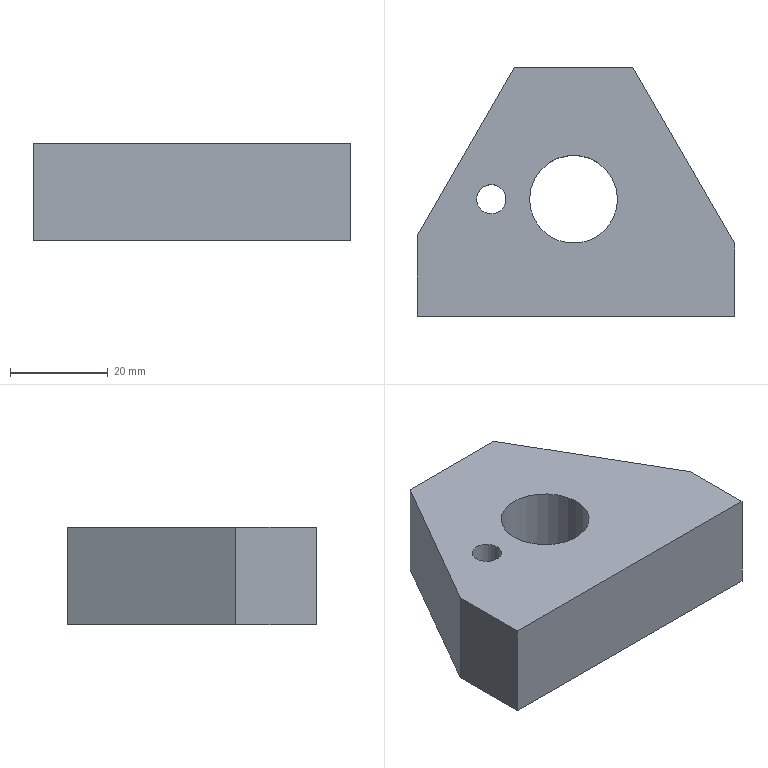NC program | NX | posted with a generic post | part box 65 x 51 x 20 mm
Whole program, first 1325 of 1400 lines:
N10 G17 G21 G94 G90
(ADAPTIVE_MILLING , TOOL : D8)
N12 T02 M6
N14 G53
N16 G17 G0 G90 X12.189 Y36.097 B0. C0. S5500 M3
N18 G43 Z30.2 H2
N20 Z3.
N22 G94 G1 X12.207 Y35.949 Z2.063 F2500.
N24 X12.226 Y35.8 Z1.692
N26 X12.244 Y35.651 Z1.42
N28 X12.263 Y35.502 Z1.2
N30 X12.282 Y35.353 Z1.016
N32 X12.3 Y35.204 Z0.858
N34 X12.319 Y35.056 Z0.72
N36 X12.338 Y34.907 Z0.6
N38 X12.356 Y34.758 Z0.495
N40 X12.375 Y34.609 Z0.402
N42 X12.393 Y34.46 Z0.321
N44 X12.412 Y34.311 Z0.25
N46 X12.431 Y34.163 Z0.19
N48 X12.449 Y34.014 Z0.138
N50 X12.468 Y33.865 Z0.095
N52 X12.487 Y33.716 Z0.061
N54 X12.505 Y33.567 Z0.034
N56 X12.524 Y33.418 Z0.015
N58 X12.542 Y33.27 Z0.004
N60 X12.561 Y33.121 Z0.
N62 X12.741 Y31.68
N64 G3 X13.293 Y31.012 R0.809
N66 X15.497 Y30.394 R12.881
N68 X21.026 Y30.043 R42.106
N70 X30.728 Y29.99 R751.289
N72 G2 X33.593 Y28.371 R4.374
N74 X35.342 Y24.592 R8.747
N76 X35.918 Y19.006 R30.143
N78 X36. Y6.781 R494.796
N80 G1 X36.013 Y-5.87
N82 X36.085 Y-6.101
N84 G2 X36.947 Y-7.722 R12.356
N86 G1 X37.005 Y-7.94
N88 G3 X36.638 Y-7.058 R3.65
N90 G2 X35.94 Y-5.799 R10.806
N92 X35.519 Y-2.949 R11.424
N94 X35.401 Y4.651 R164.559
N96 G3 X35.308 Y18.774 R515.844
N98 X34.731 Y23.984 R26.878
N100 X33.536 Y26.625 R6.339
N102 X30.052 Y28.714 R6.857
N104 X25.302 Y29.326 R21.254
N106 G2 X18.159 Y29.565 R325.443
N108 X15.126 Y29.981 R16.107
N110 X14.593 Y30.398 R2.093
N112 G1 X13.833 Y30.837
N114 G2 X15.21 Y29.843 R4.704
N116 G3 X17.513 Y28.97 R6.034
N118 X22.406 Y28.472 R34.474
N120 G2 X27.483 Y28.063 R46.592
N122 X30.66 Y26.815 R6.875
N124 X33.235 Y23.022 R8.035
N126 X34.172 Y17.947 R20.137
N128 X34.393 Y8.877 R133.127
N130 G3 X34.49 Y-1.554 R317.27
N132 X34.67 Y-3.615 R16.857
N134 X36.025 Y-5.998 R47.331
N136 G1 X34.529 Y-3.374
N138 G2 X33.982 Y-0.466 R10.299
N140 X33.799 Y7.21 R114.665
N142 G3 X33.62 Y16.757 R176.883
N144 X32.766 Y21.999 R21.482
N146 X28.366 Y26.699 R7.128
N148 X23.91 Y27.672 R17.04
N150 G2 X18.768 Y28.21 R116.087
N152 X15.92 Y29.009 R10.067
N154 G1 X15.689 Y29.199
N156 X15.19 Y29.861
N158 X15.985 Y28.817
N160 G3 X18.181 Y27.684 R5.485
N162 X22.159 Y26.925 R27.744
N164 G2 X26.35 Y26.099 R24.625
N166 X31.006 Y21.977 R7.689
N168 X32.391 Y16.852 R16.158
N170 X32.767 Y9.59 R68.766
N172 G3 X32.931 Y1.036 R215.232
N174 X33.136 Y-0.96 R18.787
N176 X34.601 Y-3.531 R124.339
N178 G1 X32.988 Y-0.707
N180 G2 X32.409 Y2.188 R10.174
N182 X32.172 Y9.2 R107.328
N184 G3 X31.756 Y16.609 R64.499
N186 X30.392 Y21.342 R14.403
N188 X26.079 Y25.131 R8.196
N190 X21.958 Y26.26 R22.038
N192 G2 X17.969 Y27.237 R27.216
N194 X16.373 Y28.082 R5.11
N196 X15.763 Y29.097 R13.29
N198 G3 X16.568 Y27.739 R54.163
N200 X18.642 Y26.378 R5.292
N202 X22.56 Y25.167 R37.442
N204 G2 X26.34 Y23.545 R12.816
N206 X29.729 Y19.042 R9.389
N208 X30.904 Y13.329 R21.33
N210 X31.243 Y5.627 R145.237
N212 G3 X31.537 Y1.832 R35.701
N214 G1 X31.591 Y1.683
N216 X33.091 Y-0.915
N218 X31.406 Y2.027
N220 G2 X30.803 Y4.924 R10.206
N222 X30.43 Y11.325 R214.4
N224 G3 X29.565 Y17.175 R28.198
N226 X26.97 Y21.765 R10.057
N228 X22.872 Y24.225 R12.042
N230 G2 X19.002 Y25.654 R134.738
N232 X17.185 Y26.687 R7.855
N234 X16.451 Y27.906 R10.718
N236 G1 X17.393 Y26.302
N238 G3 X19.431 Y24.779 R6.287
N240 G1 X22.915 Y23.099
N242 G2 X28.116 Y17.11 R10.513
N244 X29.303 Y11.315 R23.654
N246 G3 X29.808 Y5.321 R379.785
N248 X29.965 Y4.5 R3.274
N250 G1 X31.502 Y1.837
N252 X29.747 Y4.904
N254 G2 X29.095 Y7.836 R11.845
N256 G3 X28.407 Y13.239 R109.125
N258 X26.686 Y18.332 R15.466
N260 X22.682 Y22.274 R11.306
N262 X19.26 Y24.225 R480.337
N264 G2 X18.1 Y25.066 R6.557
N266 G1 X17.306 Y26.426
N268 X18.445 Y24.482
N270 G3 X20.455 Y22.697 R9.643
N272 G2 X23.549 Y20.224 R24.631
N274 X26.85 Y14.379 R13.278
N276 X27.908 Y8.936 R42.207
N278 G3 X28.158 Y7.629 R7.94
N280 G1 X29.845 Y4.706
N282 X27.9 Y8.099
N284 G2 X27.107 Y10.788 R15.997
N286 G3 X25.703 Y15.532 R28.208
N288 X21.703 Y20.822 R13.947
N290 G2 X19.443 Y22.748 R100.791
N292 G1 X18.34 Y24.633
N294 X20.078 Y21.649
N296 G3 X22.308 Y18.888 R123.62
N298 G2 X25.5 Y12.454 R19.379
N300 G1 X25.661 Y11.954
N302 X27.986 Y7.927
N304 G2 X24.49 Y14.026 R314.641
N306 G3 X22.497 Y17.434 R31.823
N308 G1 X19.984 Y21.786
N310 X24.822 Y13.407
N312 G3 X25.824 Y13.062 R0.808
N314 G1 X27.004 Y13.539
N316 X27.143 Y13.596 Z0.004
N318 X27.282 Y13.652 Z0.015
N320 X27.421 Y13.708 Z0.034
N322 X27.56 Y13.764 Z0.061
N324 X27.699 Y13.821 Z0.095
N326 X27.838 Y13.877 Z0.138
N328 X27.977 Y13.933 Z0.19
N330 X28.116 Y13.989 Z0.25
N332 X28.255 Y14.046 Z0.321
N334 X28.394 Y14.102 Z0.402
N336 X28.533 Y14.158 Z0.495
N338 X28.673 Y14.214 Z0.6
N340 X28.812 Y14.271 Z0.72
N342 X28.951 Y14.327 Z0.858
N344 X29.09 Y14.383 Z1.016
N346 X29.229 Y14.439 Z1.2
N348 X29.368 Y14.496 Z1.42
N350 X29.507 Y14.552 Z1.692
N352 X29.646 Y14.608 Z2.063
N354 X29.785 Y14.664 Z3.
N356 G0 Z30.2
N358 X42.095 Y-24.097
N360 Z3.
N362 G1 X41.946 Y-24.115 Z2.063
N364 X41.797 Y-24.133 Z1.692
N366 X41.648 Y-24.151 Z1.42
N368 X41.499 Y-24.169 Z1.2
N370 X41.35 Y-24.187 Z1.016
N372 X41.201 Y-24.205 Z0.858
N374 X41.052 Y-24.224 Z0.72
N376 X40.903 Y-24.242 Z0.6
N378 X40.754 Y-24.26 Z0.495
N380 X40.606 Y-24.278 Z0.402
N382 X40.457 Y-24.296 Z0.321
N384 X40.308 Y-24.314 Z0.25
N386 X40.159 Y-24.332 Z0.19
N388 X40.01 Y-24.35 Z0.138
N390 X39.861 Y-24.368 Z0.095
N392 X39.712 Y-24.387 Z0.061
N394 X39.563 Y-24.405 Z0.034
N396 X39.414 Y-24.423 Z0.015
N398 X39.265 Y-24.441 Z0.004
N400 X39.116 Y-24.459 Z0.
N402 X37.678 Y-24.634
N404 G3 X37.013 Y-25.169 R0.809
N406 G2 X34.462 Y-28.294 R5.205
N408 X30.179 Y-29.614 R11.739
N410 X23.443 Y-29.972 R56.241
N412 G1 X13.843 Y-30.
N414 X-29.584 Y-29.997
N416 G2 X-32.456 Y-28.549 R4.221
N418 G3 X-32.986 Y-28.077 R1.805
N420 G1 X-33.822 Y-27.784
N422 X-34.619 Y-27.284
N424 X-35.284 Y-26.619
N426 X-35.784 Y-25.822
N428 X-36.032 Y-25.114
N430 X-35.784 Y-25.822
N432 X-35.284 Y-26.619
N434 X-34.619 Y-27.284
N436 X-33.822 Y-27.784
N438 G2 X-31.94 Y-28.503 R22.769
N440 G3 X-27.671 Y-29.259 R15.645
N442 X-18.673 Y-29.398 R166.133
N444 G1 X29.268 Y-29.399
N446 G3 X32.884 Y-28.216 R21.652
N448 G1 X33.935 Y-28.095
N450 X34.822 Y-27.784
N452 X35.619 Y-27.284
N454 X36.284 Y-26.619
N456 X36.784 Y-25.822
N458 X36.284 Y-26.619
N460 X35.619 Y-27.284
N462 X34.822 Y-27.784
N464 X33.935 Y-28.095
N466 G2 X31.763 Y-28.2 R10.795
N468 X23.754 Y-28.39 R128.681
N470 G1 X16.554 Y-28.399
N472 X-28.084
N474 X-29.002 Y-28.2
N476 X-32.001
N478 X-32.935 Y-28.095
N480 X-32.001 Y-28.2
N482 X31.823
N484 G2 X32.627 Y-28.927 R0.808
N486 G1 X32.751 Y-30.156
N488 X32.766 Y-30.305 Z0.004
N490 X32.781 Y-30.454 Z0.015
N492 X32.797 Y-30.604 Z0.034
N494 X32.812 Y-30.753 Z0.061
N496 X32.827 Y-30.902 Z0.095
N498 X32.842 Y-31.051 Z0.138
N500 X32.857 Y-31.2 Z0.19
N502 X32.872 Y-31.35 Z0.25
N504 X32.887 Y-31.499 Z0.321
N506 X32.902 Y-31.648 Z0.402
N508 X32.917 Y-31.797 Z0.495
N510 X32.932 Y-31.947 Z0.6
N512 X32.947 Y-32.096 Z0.72
N514 X32.962 Y-32.245 Z0.858
N516 X32.977 Y-32.394 Z1.016
N518 X32.992 Y-32.544 Z1.2
N520 X33.008 Y-32.693 Z1.42
N522 X33.023 Y-32.842 Z1.692
N524 X33.038 Y-32.991 Z2.063
N526 X33.053 Y-33.141 Z3.
N528 G0 Z30.2
N530 X-0.084 Y-3.599
N532 Z23.
N534 G3 X-0.084 Y-3.599 Z22.605 I0.085 J3.599
N536 X-0.084 Y-3.599 Z22.21 I0.085 J3.599
N538 X-0.084 Y-3.599 Z21.816 I0.085 J3.599
N540 X-0.084 Y-3.599 Z21.421 I0.085 J3.599
N542 X-0.084 Y-3.599 Z21.026 I0.085 J3.599
N544 X-0.084 Y-3.599 Z20.631 I0.085 J3.599
N546 X-0.084 Y-3.599 Z20.236 I0.085 J3.599
N548 X-0.084 Y-3.599 Z19.841 I0.085 J3.599
N550 X-0.084 Y-3.599 Z19.447 I0.085 J3.599
N552 X-0.084 Y-3.599 Z19.052 I0.085 J3.599
N554 X-0.084 Y-3.599 Z18.657 I0.085 J3.599
N556 X-0.084 Y-3.599 Z18.262 I0.085 J3.599
N558 X-0.084 Y-3.599 Z17.867 I0.085 J3.599
N560 X-0.084 Y-3.599 Z17.472 I0.085 J3.599
N562 X-0.084 Y-3.599 Z17.078 I0.085 J3.599
N564 X-0.084 Y-3.599 Z16.683 I0.085 J3.599
N566 X-0.084 Y-3.599 Z16.288 I0.085 J3.599
N568 X-0.084 Y-3.599 Z15.893 I0.085 J3.599
N570 X-0.084 Y-3.599 Z15.498 I0.085 J3.599
N572 X-0.084 Y-3.599 Z15.104 I0.085 J3.599
N574 X-0.084 Y-3.599 Z14.709 I0.085 J3.599
N576 X-0.084 Y-3.599 Z14.314 I0.085 J3.599
N578 X-0.084 Y-3.599 Z13.919 I0.085 J3.599
N580 X-0.084 Y-3.599 Z13.524 I0.085 J3.599
N582 X-0.084 Y-3.599 Z13.129 I0.085 J3.599
N584 X-0.084 Y-3.599 Z12.735 I0.085 J3.599
N586 X-0.084 Y-3.599 Z12.34 I0.085 J3.599
N588 X-0.084 Y-3.599 Z11.945 I0.085 J3.599
N590 X-0.084 Y-3.599 Z11.55 I0.085 J3.599
N592 X-0.084 Y-3.599 Z11.155 I0.085 J3.599
N594 X-0.084 Y-3.599 Z10.76 I0.085 J3.599
N596 X-0.084 Y-3.599 Z10.366 I0.085 J3.599
N598 X-0.084 Y-3.599 Z9.971 I0.085 J3.599
N600 X-0.084 Y-3.599 Z9.576 I0.085 J3.599
N602 X-0.084 Y-3.599 Z9.181 I0.085 J3.599
N604 X-0.084 Y-3.599 Z8.786 I0.085 J3.599
N606 X-0.084 Y-3.599 Z8.392 I0.085 J3.599
N608 X-0.084 Y-3.599 Z7.997 I0.085 J3.599
N610 X-0.084 Y-3.599 Z7.602 I0.085 J3.599
N612 X-0.084 Y-3.599 Z7.207 I0.085 J3.599
N614 X-0.084 Y-3.599 Z6.812 I0.085 J3.599
N616 X-0.084 Y-3.599 Z6.417 I0.085 J3.599
N618 X-0.084 Y-3.599 Z6.023 I0.085 J3.599
N620 X-0.084 Y-3.599 Z5.628 I0.085 J3.599
N622 X-0.084 Y-3.599 Z5.233 I0.085 J3.599
N624 X-0.084 Y-3.599 Z4.838 I0.085 J3.599
N626 X-0.084 Y-3.599 Z4.443 I0.085 J3.599
N628 X-0.084 Y-3.599 Z4.048 I0.085 J3.599
N630 X-0.084 Y-3.599 Z3.654 I0.085 J3.599
N632 X-0.084 Y-3.599 Z3.259 I0.085 J3.599
N634 X-0.084 Y-3.599 Z2.864 I0.085 J3.599
N636 X-0.084 Y-3.599 Z2.469 I0.085 J3.599
N638 X-0.084 Y-3.599 Z2.074 I0.085 J3.599
N640 X-0.084 Y-3.599 Z1.679 I0.085 J3.599
N642 X-0.084 Y-3.599 Z1.285 I0.085 J3.599
N644 X-0.084 Y-3.599 Z0.89 I0.085 J3.599
N646 X-0.084 Y-3.599 Z0.495 I0.085 J3.599
N648 X-0.084 Y-3.599 Z0.1 I0.085 J3.599
N650 X3.601 Y0. Z0. R3.6
N652 X-1.005 Y-3.502 R-3.622
N654 X2.929 Y-2.208 R3.686
N656 X0.26 Y4.098 R3.798
N658 X2.236 Y-3.499 R-4.13
N660 X-0.385 Y4.617 R4.369
N662 X1.794 Y-4.328 R-4.659
N664 X4.011 Y-2.583 R5.029
N666 X4.775 Y0.391 R4.78
N668 X1.022 Y4.681 R4.849
N670 X-4.257 Y2.196 R4.846
N672 X-4.707 Y-0.888 R4.998
N674 X-2.328 Y-4.187 R4.928
N676 X2.469 Y-4.105 R4.884
N678 X4.139 Y-2.391 R4.975
N680 X3.635 Y-1.248 R0.808
N682 G1 X2.657 Y-0.975
N684 X2.512 Y-0.935 Z0.004
N686 X2.368 Y-0.895 Z0.015
N688 X2.223 Y-0.854 Z0.034
N690 X2.079 Y-0.814 Z0.061
N692 X1.934 Y-0.774 Z0.095
N694 X1.79 Y-0.734 Z0.138
N696 X1.645 Y-0.693 Z0.19
N698 X1.501 Y-0.653 Z0.25
N700 X1.356 Y-0.613 Z0.321
N702 X1.212 Y-0.572 Z0.402
N704 X1.067 Y-0.532 Z0.495
N706 X0.923 Y-0.492 Z0.6
N708 X0.778 Y-0.452 Z0.72
N710 X0.634 Y-0.411 Z0.858
N712 X0.489 Y-0.371 Z1.016
N714 X0.345 Y-0.331 Z1.2
N716 X0.201 Y-0.29 Z1.42
N718 X0.056 Y-0.25 Z1.692
N720 X-0.088 Y-0.21 Z2.063
N722 X-0.233 Y-0.17 Z3.
N724 G0 Z30.2
N726 X-41.093 Y-6.503
N728 Z3.
N730 G1 X-40.943 Y-6.512 Z2.063
N732 X-40.793 Y-6.521 Z1.692
N734 X-40.643 Y-6.529 Z1.42
N736 X-40.494 Y-6.538 Z1.2
N738 X-40.344 Y-6.547 Z1.016
N740 X-40.194 Y-6.555 Z0.858
N742 X-40.044 Y-6.564 Z0.72
N744 X-39.895 Y-6.573 Z0.6
N746 X-39.745 Y-6.581 Z0.495
N748 X-39.595 Y-6.59 Z0.402
N750 X-39.445 Y-6.599 Z0.321
N752 X-39.296 Y-6.607 Z0.25
N754 X-39.146 Y-6.616 Z0.19
N756 X-38.996 Y-6.625 Z0.138
N758 X-38.846 Y-6.633 Z0.095
N760 X-38.697 Y-6.642 Z0.061
N762 X-38.547 Y-6.651 Z0.034
N764 X-38.397 Y-6.659 Z0.015
N766 X-38.247 Y-6.668 Z0.004
N768 X-38.098 Y-6.677 Z0.
N770 X-36.818 Y-6.751
N772 G3 X-35.991 Y-6.153 R0.808
N774 G2 X-35.712 Y-5.458 R6.604
N776 G3 X-35.172 Y-2.041 R14.267
N778 X-35.003 Y7.056 R159.941
N780 G1 X-35. Y10.354
N782 X-34.999 Y24.529
N784 G2 X-33.477 Y27.518 R4.216
N786 X-29.801 Y29.298 R8.415
N788 X-24.294 Y29.909 R28.12
N790 X-15.23 Y30.014 R512.471
N792 G3 X-14.593 Y30.398 R1.168
N794 G1 X-13.833 Y30.837
N796 X-13.262 Y31.022
N798 G3 X-14.992 Y30.046 R3.953
N800 G2 X-17.002 Y29.599 R6.273
N802 X-23.088 Y29.34 R96.329
N804 G3 X-28.533 Y28.838 R33.359
N806 X-31.258 Y27.823 R7.63
N808 X-33.556 Y24.574 R6.295
N810 X-34.283 Y20.072 R17.047
N812 X-34.399 Y11.523 R188.539
N814 G2 X-34.517 Y-0.552 R326.859
N816 X-34.859 Y-3.942 R24.382
N818 X-35.637 Y-5.325 R24.387
N820 G1 X-35.764 Y-5.597
N822 G2 X-34.44 Y-3.231 R50.341
N824 G3 X-33.697 Y0.105 R11.455
N826 X-33.417 Y7.598 R85.64
N828 G2 X-33.324 Y18.309 R463.198
N830 X-32.785 Y22.691 R19.446
N832 X-29.728 Y26.458 R6.318
N834 X-25.039 Y27.949 R13.182
N836 X-19.274 Y28.441 R70.147
N838 G3 X-16.066 Y28.906 R15.148
N840 X-15.72 Y29.158 R1.377
N842 G2 X-14.911 Y30.111 R3.9
N844 G3 X-15.72 Y29.158 R3.9
N846 G2 X-16.552 Y28.584 R1.688
N848 X-19.977 Y27.889 R13.765
N850 G3 X-25.031 Y27.277 R68.554
N852 X-28.896 Y25.906 R11.131
N854 X-31.797 Y22.061 R7.297
N856 X-32.645 Y17.275 R17.933
N858 X-32.808 Y9.069 R154.48
N860 G2 X-33.075 Y0.798 R101.196
N862 X-33.437 Y-1.506 R15.46
N864 G1 X-34.504 Y-3.362
N866 X-32.903 Y-0.563
N868 G3 X-32.112 Y3.027 R12.495
N870 X-31.818 Y10.092 R84.199
N872 G2 X-31.569 Y17.36 R93.163
N874 X-30.639 Y21.36 R12.888
N876 X-26.856 Y25.069 R7.753
N878 X-22.271 Y26.44 R17.487
N880 G3 X-18.139 Y27.214 R62.228
N882 X-16.554 Y27.826 R5.011
N884 G1 X-16.398 Y27.997
N886 X-15.761 Y29.101
N888 X-16.473 Y27.868
N890 G2 X-18.044 Y26.912 R3.739
N892 X-21.722 Y25.965 R28.639
N894 G3 X-25.999 Y24.607 R18.26
N896 X-30.111 Y19.852 R8.111
N898 X-31.037 Y14.701 R19.369
N900 X-31.285 Y7.063 R249.753
N902 G2 X-31.806 Y1.483 R35.469
N904 G1 X-31.905 Y1.138
N906 X-32.993 Y-0.745
N908 X-31.357 Y2.109
N910 G3 X-30.543 Y5.61 R12.165
N912 X-30.14 Y12.497 R111.252
N914 G2 X-29.483 Y17.696 R26.095
N916 X-24.975 Y23.375 R8.64
N918 X-21.427 Y24.794 R20.567
N920 G3 X-17.901 Y26.048 R26.491
N922 X-17.259 Y26.506 R1.514
N924 G1 X-16.472 Y27.87
N926 X-17.375 Y26.313
N928 G2 X-19.253 Y25.093 R5.396
N930 G1 X-22.84 Y23.643
N932 G3 X-26.735 Y20.912 R10.468
N934 X-28.95 Y16.128 R10.9
N936 X-29.603 Y10.396 R37.582
N938 G2 X-30.149 Y4.597 R49.593
N940 X-30.317 Y3.89 R8.507
N942 G1 X-31.442 Y1.941
N944 X-29.736 Y4.919
N946 G3 X-28.901 Y8.439 R13.323
N948 G2 X-28.282 Y13.719 R208.993
N950 X-26.909 Y18.136 R13.401
N952 X-23.191 Y21.884 R10.319
N954 X-19.652 Y23.773 R52.367
N956 G3 X-18.46 Y24.489 R9.25
N958 G1 X-18.348 Y24.621
N960 X-17.298 Y26.439
N962 G2 X-18.532 Y24.346 R33.435
N964 X-20.505 Y22.838 R8.687
N966 G3 X-23.867 Y20.516 R24.146
N968 X-27.186 Y14.987 R11.101
N970 X-28.096 Y9.925 R37.28
N972 G2 X-28.64 Y6.808 R29.229
N974 G1 X-29.794 Y4.796
N976 G3 X-27.987 Y7.971 R68.743
N978 X-27.096 Y11. R17.792
N980 G2 X-25.832 Y15.396 R26.405
N982 X-22.068 Y20.247 R12.322
N984 G1 X-19.905 Y21.955
N986 G3 X-18.413 Y24.508 R264.636
N988 G1 X-20.089 Y21.634
N990 G2 X-22.027 Y19.562 R24.886
N992 G3 X-24.309 Y16.624 R15.109
N994 G1 X-27.114 Y11.766
N996 G2 X-27.477 Y11.419 R1.104
N998 G1 X-28.752 Y10.511 Z0.1
N1000 X-29.103 Y10.258 F15000.
N1002 X-29.463 Y10.016
N1004 G2 X-30.163 Y10.006 R0.802
N1006 G1 X-30.439 Y10.137
N1008 X-30.721 Y10.255
N1010 G3 X-31.365 Y8.81 R0.8
N1012 G1 X-30.19 Y8.059
N1014 X-29.667 Y7.72 Z0.06 F2500.
N1016 X-29.137 Y7.394 Z0.02
N1018 X-28.986 Y7.343 Z0.01
N1020 X-28.829 Y7.319 Z0.
N1022 G3 X-28.106 Y7.719 R0.801
N1024 X-25.688 Y12.114 R88.793
N1026 G2 X-23.187 Y16.322 R42.88
N1028 G1 X-22.953 Y16.644
N1030 X-19.953 Y21.84
N1032 X-26.928 Y9.759
N1034 G2 X-27.931 Y9.414 R0.808
N1036 G1 X-29.11 Y9.891
N1038 X-29.249 Y9.947 Z0.004
N1040 X-29.388 Y10.004 Z0.015
N1042 X-29.527 Y10.06 Z0.034
N1044 X-29.666 Y10.116 Z0.061
N1046 X-29.806 Y10.172 Z0.095
N1048 X-29.945 Y10.229 Z0.138
N1050 X-30.084 Y10.285 Z0.19
N1052 X-30.223 Y10.341 Z0.25
N1054 X-30.362 Y10.397 Z0.321
N1056 X-30.501 Y10.454 Z0.402
N1058 X-30.64 Y10.51 Z0.495
N1060 X-30.779 Y10.566 Z0.6
N1062 X-30.918 Y10.622 Z0.72
N1064 X-31.057 Y10.679 Z0.858
N1066 X-31.196 Y10.735 Z1.016
N1068 X-31.335 Y10.791 Z1.2
N1070 X-31.474 Y10.847 Z1.42
N1072 X-31.613 Y10.904 Z1.692
N1074 X-31.752 Y10.96 Z2.063
N1076 X-31.891 Y11.016 Z3.
N1078 G0 Z30.2
(PLANAR_MILL_COPY , TOOL : D8)
N1080 X-3.98 Y0.413 S4500
N1082 Z30.
N1084 Z3.
N1086 G1 Z0. F600.
N1088 G41 X-4.472 Y0.5 D2
N1090 X-4.5
N1092 G3 X-5. Y0. R0.5
N1094 X0. Y-5. R5.
N1096 X-5. Y0. R-5.
N1098 X-4.472 Y-0.5 R0.501
N1100 G40
N1102 G1 X-3.98 Y-0.413
N1104 Z3.
N1106 G0 Z30.
(PLANAR_MILL , TOOL : D8)
N1108 X0.5 Y-31.9
N1110 Z3.
N1112 G1 Z0.
N1114 Y-27.9
N1116 X-31.9
N1118 G2 X-35.9 Y-23.9 R4.
N1120 G1 Y-7.452
N1122 G2 X-35.364 Y-5.452 R4.
N1124 G1 X-15.531 Y28.9
N1126 G2 X-12.067 Y30.9 R4.
N1128 G1 X12.067
N1130 G2 X15.531 Y28.9 R4.
N1132 G1 X36.364 Y-7.184
N1134 G2 X36.9 Y-9.184 R4.
N1136 G1 Y-23.9
N1138 G2 X32.9 Y-27.9 R4.
N1140 G1 X0.5
N1142 Y-31.9
N1144 Z3.
N1146 G0 Z30.
(DRILLING , TOOL : D8)
N1148 S0
N1150 X-16.85 Y0.
N1152 G43 Z23. H2
N1154 G81 G99 Z20. F250. R23.
N1156 G80
N1158 M5
(PLANAR_MILL_1 , TOOL : D4平刀)
N1160 T12 M6
N1162 G54
N1164 G17 G43 G0 G90 X-31.162 Y-0.338 B0. C0. S3500 H12 M3
N1166 Z0.5
N1168 G94 G1 X-31.093 Y-0.944 Z0.489 F500.
N1170 X-30.702 Y-1.448 Z0.478
N1172 X-30.106 Y-1.675 Z0.467
N1174 X-29.582 Y-1.603 Z0.458
N1176 X-29.035 Y-1.179 Z0.446
N1178 X-28.835 Y-0.69 Z0.437
N1180 X-28.929 Y-0.004 Z0.424
N1182 X-29.253 Y0.414 Z0.415
N1184 X-29.838 Y0.669 Z0.404
N1186 X-30.47 Y0.582 Z0.393
N1188 X-30.965 Y0.179 Z0.382
N1190 X-31.165 Y-0.31 Z0.373
N1192 X-31.093 Y-0.944 Z0.361
N1194 X-30.702 Y-1.448 Z0.35
N1196 X-30.106 Y-1.675 Z0.339
N1198 X-29.582 Y-1.603 Z0.33
N1200 X-29.035 Y-1.179 Z0.318
N1202 X-28.835 Y-0.69 Z0.309
N1204 X-28.929 Y-0.004 Z0.297
N1206 X-29.253 Y0.414 Z0.287
N1208 X-29.838 Y0.669 Z0.276
N1210 X-30.47 Y0.582 Z0.265
N1212 X-30.965 Y0.179 Z0.254
N1214 X-31.165 Y-0.31 Z0.245
N1216 X-31.093 Y-0.944 Z0.234
N1218 X-30.702 Y-1.448 Z0.222
N1220 X-30.106 Y-1.675 Z0.211
N1222 X-29.582 Y-1.603 Z0.202
N1224 X-29.035 Y-1.179 Z0.19
N1226 X-28.835 Y-0.69 Z0.181
N1228 X-28.929 Y-0.004 Z0.169
N1230 X-29.253 Y0.414 Z0.159
N1232 X-29.838 Y0.669 Z0.148
N1234 X-30.47 Y0.582 Z0.137
N1236 X-30.965 Y0.179 Z0.126
N1238 X-31.165 Y-0.31 Z0.117
N1240 X-31.093 Y-0.944 Z0.106
N1242 X-30.702 Y-1.448 Z0.095
N1244 X-30.106 Y-1.675 Z0.083
N1246 X-29.582 Y-1.603 Z0.074
N1248 X-29.035 Y-1.179 Z0.062
N1250 X-28.835 Y-0.69 Z0.053
N1252 X-28.929 Y-0.004 Z0.041
N1254 X-29.253 Y0.414 Z0.032
N1256 X-29.838 Y0.669 Z0.02
N1258 X-30.47 Y0.582 Z0.009
N1260 X-30.965 Y0.179 Z-0.002
N1262 X-31.165 Y-0.31 Z-0.011
N1264 X-31.093 Y-0.944 Z-0.022
N1266 X-30.702 Y-1.448 Z-0.033
N1268 X-30.106 Y-1.675 Z-0.045
N1270 X-29.582 Y-1.603 Z-0.054
N1272 X-29.035 Y-1.179 Z-0.066
N1274 X-28.835 Y-0.69 Z-0.075
N1276 X-28.929 Y-0.004 Z-0.087
N1278 X-29.253 Y0.414 Z-0.096
N1280 X-29.838 Y0.669 Z-0.107
N1282 X-30.47 Y0.582 Z-0.119
N1284 X-30.965 Y0.179 Z-0.13
N1286 X-31.165 Y-0.31 Z-0.139
N1288 X-31.093 Y-0.944 Z-0.15
N1290 X-30.702 Y-1.448 Z-0.161
N1292 X-30.106 Y-1.675 Z-0.172
N1294 X-29.582 Y-1.603 Z-0.182
N1296 X-29.035 Y-1.179 Z-0.194
N1298 X-28.835 Y-0.69 Z-0.203
N1300 X-28.929 Y-0.004 Z-0.215
N1302 X-29.253 Y0.414 Z-0.224
N1304 X-29.838 Y0.669 Z-0.235
N1306 X-30.47 Y0.582 Z-0.247
N1308 X-30.965 Y0.179 Z-0.258
N1310 X-31.165 Y-0.31 Z-0.267
N1312 X-31.093 Y-0.944 Z-0.278
N1314 X-30.702 Y-1.448 Z-0.289
N1316 X-30.106 Y-1.675 Z-0.3
N1318 X-29.582 Y-1.603 Z-0.31
N1320 X-29.035 Y-1.179 Z-0.322
N1322 X-28.835 Y-0.69 Z-0.331
N1324 X-28.929 Y-0.004 Z-0.343
N1326 X-29.253 Y0.414 Z-0.352
N1328 X-29.838 Y0.669 Z-0.363
N1330 X-30.47 Y0.582 Z-0.374
N1332 X-30.965 Y0.179 Z-0.386
N1334 X-31.165 Y-0.31 Z-0.395
N1336 X-31.093 Y-0.944 Z-0.406
N1338 X-30.702 Y-1.448 Z-0.417
N1340 X-30.106 Y-1.675 Z-0.428
N1342 X-29.582 Y-1.603 Z-0.437
N1344 X-29.035 Y-1.179 Z-0.45
N1346 X-28.835 Y-0.69 Z-0.459
N1348 X-28.929 Y-0.004 Z-0.471
N1350 X-29.253 Y0.414 Z-0.48
N1352 X-29.838 Y0.669 Z-0.491
N1354 X-30.47 Y0.582 Z-0.502
N1356 X-30.965 Y0.179 Z-0.513
N1358 X-31.165 Y-0.31 Z-0.523
N1360 X-31.093 Y-0.944 Z-0.534
N1362 X-30.702 Y-1.448 Z-0.545
N1364 X-30.106 Y-1.675 Z-0.556
N1366 X-29.582 Y-1.603 Z-0.565
N1368 X-29.035 Y-1.179 Z-0.577
N1370 X-28.835 Y-0.69 Z-0.587
N1372 X-28.929 Y-0.004 Z-0.599
N1374 X-29.253 Y0.414 Z-0.608
N1376 X-29.838 Y0.669 Z-0.619
N1378 X-30.47 Y0.582 Z-0.63
N1380 X-30.965 Y0.179 Z-0.641
N1382 X-31.165 Y-0.31 Z-0.651
N1384 X-31.093 Y-0.944 Z-0.662
N1386 X-30.702 Y-1.448 Z-0.673
N1388 X-30.106 Y-1.675 Z-0.684
N1390 X-29.582 Y-1.603 Z-0.693
N1392 X-29.035 Y-1.179 Z-0.705
N1394 X-28.835 Y-0.69 Z-0.715
N1396 X-28.929 Y-0.004 Z-0.727
N1398 X-29.253 Y0.414 Z-0.736
N1400 X-29.838 Y0.669 Z-0.747
N1402 X-30.47 Y0.582 Z-0.758
N1404 X-30.965 Y0.179 Z-0.769
N1406 X-31.165 Y-0.31 Z-0.778
N1408 X-31.093 Y-0.944 Z-0.79
N1410 X-30.702 Y-1.448 Z-0.801
N1412 X-30.106 Y-1.675 Z-0.812
N1414 X-29.582 Y-1.603 Z-0.821
N1416 X-29.035 Y-1.179 Z-0.833
N1418 X-28.835 Y-0.69 Z-0.842
N1420 X-28.929 Y-0.004 Z-0.855
N1422 X-29.253 Y0.414 Z-0.864
N1424 X-29.838 Y0.669 Z-0.875
N1426 X-30.47 Y0.582 Z-0.886
N1428 X-30.965 Y0.179 Z-0.897
N1430 X-31.165 Y-0.31 Z-0.906
N1432 X-31.093 Y-0.944 Z-0.918
N1434 X-30.702 Y-1.448 Z-0.929
N1436 X-30.106 Y-1.675 Z-0.94
N1438 X-29.582 Y-1.603 Z-0.949
N1440 X-29.035 Y-1.179 Z-0.961
N1442 X-28.835 Y-0.69 Z-0.97
N1444 X-28.929 Y-0.004 Z-0.982
N1446 X-29.253 Y0.414 Z-0.992
N1448 X-29.838 Y0.669 Z-1.003
N1450 X-30.47 Y0.582 Z-1.014
N1452 X-30.965 Y0.179 Z-1.025
N1454 X-31.165 Y-0.31 Z-1.034
N1456 X-31.093 Y-0.944 Z-1.045
N1458 X-30.702 Y-1.448 Z-1.057
N1460 X-30.106 Y-1.675 Z-1.068
N1462 X-29.582 Y-1.603 Z-1.077
N1464 X-29.035 Y-1.179 Z-1.089
N1466 X-28.835 Y-0.69 Z-1.098
N1468 X-28.929 Y-0.004 Z-1.11
N1470 X-29.253 Y0.414 Z-1.12
N1472 X-29.838 Y0.669 Z-1.131
N1474 X-30.47 Y0.582 Z-1.142
N1476 X-30.965 Y0.179 Z-1.153
N1478 X-31.165 Y-0.31 Z-1.162
N1480 X-31.093 Y-0.944 Z-1.173
N1482 X-30.702 Y-1.448 Z-1.184
N1484 X-30.106 Y-1.675 Z-1.196
N1486 X-29.582 Y-1.603 Z-1.205
N1488 X-29.035 Y-1.179 Z-1.217
N1490 X-28.835 Y-0.69 Z-1.226
N1492 X-28.929 Y-0.004 Z-1.238
N1494 X-29.253 Y0.414 Z-1.247
N1496 X-29.838 Y0.669 Z-1.259
N1498 X-30.47 Y0.582 Z-1.27
N1500 X-30.965 Y0.179 Z-1.281
N1502 X-31.165 Y-0.31 Z-1.29
N1504 X-31.093 Y-0.944 Z-1.301
N1506 X-30.702 Y-1.448 Z-1.312
N1508 X-30.106 Y-1.675 Z-1.323
N1510 X-29.582 Y-1.603 Z-1.333
N1512 X-29.035 Y-1.179 Z-1.345
N1514 X-28.835 Y-0.69 Z-1.354
N1516 X-28.929 Y-0.004 Z-1.366
N1518 X-29.253 Y0.414 Z-1.375
N1520 X-29.838 Y0.669 Z-1.386
N1522 X-30.47 Y0.582 Z-1.398
N1524 X-30.965 Y0.179 Z-1.409
N1526 X-31.165 Y-0.31 Z-1.418
N1528 X-31.093 Y-0.944 Z-1.429
N1530 X-30.702 Y-1.448 Z-1.44
N1532 X-30.106 Y-1.675 Z-1.451
N1534 X-29.582 Y-1.603 Z-1.461
N1536 X-29.035 Y-1.179 Z-1.473
N1538 X-28.835 Y-0.69 Z-1.482
N1540 X-28.929 Y-0.004 Z-1.494
N1542 X-29.253 Y0.414 Z-1.503
N1544 X-29.838 Y0.669 Z-1.514
N1546 X-30.47 Y0.582 Z-1.525
N1548 X-30.965 Y0.179 Z-1.537
N1550 X-31.165 Y-0.31 Z-1.546
N1552 X-31.093 Y-0.944 Z-1.557
N1554 X-30.702 Y-1.448 Z-1.568
N1556 X-30.106 Y-1.675 Z-1.579
N1558 X-29.582 Y-1.603 Z-1.588
N1560 X-29.035 Y-1.179 Z-1.601
N1562 X-28.835 Y-0.69 Z-1.61
N1564 X-28.929 Y-0.004 Z-1.622
N1566 X-29.253 Y0.414 Z-1.631
N1568 X-29.838 Y0.669 Z-1.642
N1570 X-30.47 Y0.582 Z-1.653
N1572 X-30.965 Y0.179 Z-1.665
N1574 X-31.165 Y-0.31 Z-1.674
N1576 X-31.093 Y-0.944 Z-1.685
N1578 X-30.702 Y-1.448 Z-1.696
N1580 X-30.106 Y-1.675 Z-1.707
N1582 X-29.582 Y-1.603 Z-1.716
N1584 X-29.035 Y-1.179 Z-1.728
N1586 X-28.835 Y-0.69 Z-1.738
N1588 X-28.929 Y-0.004 Z-1.75
N1590 X-29.253 Y0.414 Z-1.759
N1592 X-29.838 Y0.669 Z-1.77
N1594 X-30.47 Y0.582 Z-1.781
N1596 X-30.965 Y0.179 Z-1.792
N1598 X-31.165 Y-0.31 Z-1.802
N1600 X-31.093 Y-0.944 Z-1.813
N1602 X-30.702 Y-1.448 Z-1.824
N1604 X-30.106 Y-1.675 Z-1.835
N1606 X-29.582 Y-1.603 Z-1.844
N1608 X-29.035 Y-1.179 Z-1.856
N1610 X-28.835 Y-0.69 Z-1.866
N1612 X-28.929 Y-0.004 Z-1.878
N1614 X-29.253 Y0.414 Z-1.887
N1616 X-29.838 Y0.669 Z-1.898
N1618 X-30.47 Y0.582 Z-1.909
N1620 X-30.965 Y0.179 Z-1.92
N1622 X-31.165 Y-0.31 Z-1.93
N1624 X-31.093 Y-0.944 Z-1.941
N1626 X-30.702 Y-1.448 Z-1.952
N1628 X-30.106 Y-1.675 Z-1.963
N1630 X-29.582 Y-1.603 Z-1.972
N1632 X-29.035 Y-1.179 Z-1.984
N1634 X-28.835 Y-0.69 Z-1.993
N1636 X-28.929 Y-0.004 Z-2.006
N1638 X-29.253 Y0.414 Z-2.015
N1640 X-29.838 Y0.669 Z-2.026
N1642 X-30.47 Y0.582 Z-2.037
N1644 X-30.965 Y0.179 Z-2.048
N1646 X-31.165 Y-0.31 Z-2.057
N1648 X-31.093 Y-0.944 Z-2.069
N1650 X-30.702 Y-1.448 Z-2.08
N1652 X-30.106 Y-1.675 Z-2.091
N1654 X-29.582 Y-1.603 Z-2.1
N1656 X-29.035 Y-1.179 Z-2.112
N1658 X-28.835 Y-0.69 Z-2.121
N1660 X-28.929 Y-0.004 Z-2.133
N1662 X-29.253 Y0.414 Z-2.143
N1664 X-29.838 Y0.669 Z-2.154
N1666 X-30.47 Y0.582 Z-2.165
N1668 X-30.965 Y0.179 Z-2.176
N1670 X-31.165 Y-0.31 Z-2.185
N1672 X-31.093 Y-0.944 Z-2.196
N1674 X-30.702 Y-1.448 Z-2.208
N1676 X-30.106 Y-1.675 Z-2.219
N1678 X-29.582 Y-1.603 Z-2.228
N1680 X-29.035 Y-1.179 Z-2.24
N1682 X-28.835 Y-0.69 Z-2.249
N1684 X-28.929 Y-0.004 Z-2.261
N1686 X-29.253 Y0.414 Z-2.271
N1688 X-29.838 Y0.669 Z-2.282
N1690 X-30.47 Y0.582 Z-2.293
N1692 X-30.965 Y0.179 Z-2.304
N1694 X-31.165 Y-0.31 Z-2.313
N1696 X-31.093 Y-0.944 Z-2.324
N1698 X-30.702 Y-1.448 Z-2.336
N1700 X-30.106 Y-1.675 Z-2.347
N1702 X-29.582 Y-1.603 Z-2.356
N1704 X-29.035 Y-1.179 Z-2.368
N1706 X-28.835 Y-0.69 Z-2.377
N1708 X-28.929 Y-0.004 Z-2.389
N1710 X-29.253 Y0.414 Z-2.398
N1712 X-29.838 Y0.669 Z-2.41
N1714 X-30.47 Y0.582 Z-2.421
N1716 X-30.965 Y0.179 Z-2.432
N1718 X-31.165 Y-0.31 Z-2.441
N1720 X-31.093 Y-0.944 Z-2.452
N1722 X-30.702 Y-1.448 Z-2.463
N1724 X-30.106 Y-1.675 Z-2.475
N1726 X-29.582 Y-1.603 Z-2.484
N1728 X-29.035 Y-1.179 Z-2.496
N1730 X-28.835 Y-0.69 Z-2.505
N1732 X-28.929 Y-0.004 Z-2.517
N1734 X-29.253 Y0.414 Z-2.526
N1736 X-29.838 Y0.669 Z-2.538
N1738 X-30.47 Y0.582 Z-2.549
N1740 X-30.965 Y0.179 Z-2.56
N1742 X-31.165 Y-0.31 Z-2.569
N1744 X-31.093 Y-0.944 Z-2.58
N1746 X-30.702 Y-1.448 Z-2.591
N1748 X-30.106 Y-1.675 Z-2.602
N1750 X-29.582 Y-1.603 Z-2.612
N1752 X-29.035 Y-1.179 Z-2.624
N1754 X-28.835 Y-0.69 Z-2.633
N1756 X-28.929 Y-0.004 Z-2.645
N1758 X-29.253 Y0.414 Z-2.654
N1760 X-29.838 Y0.669 Z-2.665
N1762 X-30.47 Y0.582 Z-2.677
N1764 X-30.965 Y0.179 Z-2.688
N1766 X-31.165 Y-0.31 Z-2.697
N1768 X-31.093 Y-0.944 Z-2.708
N1770 X-30.702 Y-1.448 Z-2.719
N1772 X-30.106 Y-1.675 Z-2.73
N1774 X-29.582 Y-1.603 Z-2.74
N1776 X-29.035 Y-1.179 Z-2.752
N1778 X-28.835 Y-0.69 Z-2.761
N1780 X-28.929 Y-0.004 Z-2.773
N1782 X-29.253 Y0.414 Z-2.782
N1784 X-29.838 Y0.669 Z-2.793
N1786 X-30.47 Y0.582 Z-2.804
N1788 X-30.965 Y0.179 Z-2.816
N1790 X-31.165 Y-0.31 Z-2.825
N1792 X-31.093 Y-0.944 Z-2.836
N1794 X-30.702 Y-1.448 Z-2.847
N1796 X-30.106 Y-1.675 Z-2.858
N1798 X-29.582 Y-1.603 Z-2.867
N1800 X-29.035 Y-1.179 Z-2.88
N1802 X-28.835 Y-0.69 Z-2.889
N1804 X-28.929 Y-0.004 Z-2.901
N1806 X-29.253 Y0.414 Z-2.91
N1808 X-29.838 Y0.669 Z-2.921
N1810 X-30.47 Y0.582 Z-2.932
N1812 X-30.965 Y0.179 Z-2.943
N1814 X-31.165 Y-0.31 Z-2.953
N1816 X-31.093 Y-0.944 Z-2.964
N1818 X-30.702 Y-1.448 Z-2.975
N1820 X-30.106 Y-1.675 Z-2.986
N1822 X-29.582 Y-1.603 Z-2.995
N1824 X-29.035 Y-1.179 Z-3.007
N1826 X-28.835 Y-0.69 Z-3.017
N1828 X-28.929 Y-0.004 Z-3.029
N1830 X-29.253 Y0.414 Z-3.038
N1832 X-29.838 Y0.669 Z-3.049
N1834 X-30.47 Y0.582 Z-3.06
N1836 X-30.965 Y0.179 Z-3.071
N1838 X-31.165 Y-0.31 Z-3.081
N1840 X-31.093 Y-0.944 Z-3.092
N1842 X-30.702 Y-1.448 Z-3.103
N1844 X-30.106 Y-1.675 Z-3.114
N1846 X-29.582 Y-1.603 Z-3.123
N1848 X-29.035 Y-1.179 Z-3.135
N1850 X-28.835 Y-0.69 Z-3.145
N1852 X-28.929 Y-0.004 Z-3.157
N1854 X-29.253 Y0.414 Z-3.166
N1856 X-29.838 Y0.669 Z-3.177
N1858 X-30.47 Y0.582 Z-3.188
N1860 X-30.965 Y0.179 Z-3.199
N1862 X-31.165 Y-0.31 Z-3.209
N1864 X-31.093 Y-0.944 Z-3.22
N1866 X-30.702 Y-1.448 Z-3.231
N1868 X-30.106 Y-1.675 Z-3.242
N1870 X-29.582 Y-1.603 Z-3.251
N1872 X-29.035 Y-1.179 Z-3.263
N1874 X-28.835 Y-0.69 Z-3.272
N1876 X-28.929 Y-0.004 Z-3.285
N1878 X-29.253 Y0.414 Z-3.294
N1880 X-29.838 Y0.669 Z-3.305
N1882 X-30.47 Y0.582 Z-3.316
N1884 X-30.965 Y0.179 Z-3.327
N1886 X-31.165 Y-0.31 Z-3.336
N1888 X-31.093 Y-0.944 Z-3.348
N1890 X-30.702 Y-1.448 Z-3.359
N1892 X-30.106 Y-1.675 Z-3.37
N1894 X-29.582 Y-1.603 Z-3.379
N1896 X-29.035 Y-1.179 Z-3.391
N1898 X-28.835 Y-0.69 Z-3.4
N1900 X-28.929 Y-0.004 Z-3.412
N1902 X-29.253 Y0.414 Z-3.422
N1904 X-29.838 Y0.669 Z-3.433
N1906 X-30.47 Y0.582 Z-3.444
N1908 X-30.965 Y0.179 Z-3.455
N1910 X-31.165 Y-0.31 Z-3.464
N1912 X-31.093 Y-0.944 Z-3.475
N1914 X-30.702 Y-1.448 Z-3.487
N1916 X-30.106 Y-1.675 Z-3.498
N1918 X-29.582 Y-1.603 Z-3.507
N1920 X-29.035 Y-1.179 Z-3.519
N1922 X-28.835 Y-0.69 Z-3.528
N1924 X-28.929 Y-0.004 Z-3.54
N1926 X-29.253 Y0.414 Z-3.55
N1928 X-29.838 Y0.669 Z-3.561
N1930 X-30.47 Y0.582 Z-3.572
N1932 X-30.965 Y0.179 Z-3.583
N1934 X-31.165 Y-0.31 Z-3.592
N1936 X-31.093 Y-0.944 Z-3.603
N1938 X-30.702 Y-1.448 Z-3.614
N1940 X-30.106 Y-1.675 Z-3.626
N1942 X-29.582 Y-1.603 Z-3.635
N1944 X-29.035 Y-1.179 Z-3.647
N1946 X-28.835 Y-0.69 Z-3.656
N1948 X-28.929 Y-0.004 Z-3.668
N1950 X-29.253 Y0.414 Z-3.677
N1952 X-29.838 Y0.669 Z-3.689
N1954 X-30.47 Y0.582 Z-3.7
N1956 X-30.965 Y0.179 Z-3.711
N1958 X-31.165 Y-0.31 Z-3.72
N1960 X-31.093 Y-0.944 Z-3.731
N1962 X-30.702 Y-1.448 Z-3.742
N1964 X-30.106 Y-1.675 Z-3.753
N1966 X-29.582 Y-1.603 Z-3.763
N1968 X-29.035 Y-1.179 Z-3.775
N1970 X-28.835 Y-0.69 Z-3.784
N1972 X-28.929 Y-0.004 Z-3.796
N1974 X-29.253 Y0.414 Z-3.805
N1976 X-29.838 Y0.669 Z-3.816
N1978 X-30.47 Y0.582 Z-3.828
N1980 X-30.965 Y0.179 Z-3.839
N1982 X-31.165 Y-0.31 Z-3.848
N1984 X-31.093 Y-0.944 Z-3.859
N1986 X-30.702 Y-1.448 Z-3.87
N1988 X-30.106 Y-1.675 Z-3.881
N1990 X-29.582 Y-1.603 Z-3.891
N1992 X-29.035 Y-1.179 Z-3.903
N1994 X-28.835 Y-0.69 Z-3.912
N1996 X-28.929 Y-0.004 Z-3.924
N1998 X-29.253 Y0.414 Z-3.933
N2000 X-29.838 Y0.669 Z-3.944
N2002 X-30.47 Y0.582 Z-3.956
N2004 X-30.965 Y0.179 Z-3.967
N2006 X-31.165 Y-0.31 Z-3.976
N2008 X-31.093 Y-0.944 Z-3.987
N2010 X-30.702 Y-1.448 Z-3.998
N2012 X-30.106 Y-1.675 Z-4.009
N2014 X-29.582 Y-1.603 Z-4.019
N2016 X-29.035 Y-1.179 Z-4.031
N2018 X-28.835 Y-0.69 Z-4.04
N2020 X-28.929 Y-0.004 Z-4.052
N2022 X-29.253 Y0.414 Z-4.061
N2024 X-29.838 Y0.669 Z-4.072
N2026 X-30.47 Y0.582 Z-4.083
N2028 X-30.965 Y0.179 Z-4.095
N2030 X-31.165 Y-0.31 Z-4.104
N2032 X-31.093 Y-0.944 Z-4.115
N2034 X-30.702 Y-1.448 Z-4.126
N2036 X-30.106 Y-1.675 Z-4.137
N2038 X-29.582 Y-1.603 Z-4.146
N2040 X-29.035 Y-1.179 Z-4.158
N2042 X-28.835 Y-0.69 Z-4.168
N2044 X-28.929 Y-0.004 Z-4.18
N2046 X-29.253 Y0.414 Z-4.189
N2048 X-29.838 Y0.669 Z-4.2
N2050 X-30.47 Y0.582 Z-4.211
N2052 X-30.965 Y0.179 Z-4.222
N2054 X-31.165 Y-0.31 Z-4.232
N2056 X-31.093 Y-0.944 Z-4.243
N2058 X-30.702 Y-1.448 Z-4.254
N2060 X-30.106 Y-1.675 Z-4.265
N2062 X-29.582 Y-1.603 Z-4.274
N2064 X-29.035 Y-1.179 Z-4.286
N2066 X-28.835 Y-0.69 Z-4.296
N2068 X-28.929 Y-0.004 Z-4.308
N2070 X-29.253 Y0.414 Z-4.317
N2072 X-29.838 Y0.669 Z-4.328
N2074 X-30.47 Y0.582 Z-4.339
N2076 X-30.965 Y0.179 Z-4.35
N2078 X-31.165 Y-0.31 Z-4.36
N2080 X-31.093 Y-0.944 Z-4.371
N2082 X-30.702 Y-1.448 Z-4.382
N2084 X-30.106 Y-1.675 Z-4.393
N2086 X-29.582 Y-1.603 Z-4.402
N2088 X-29.035 Y-1.179 Z-4.414
N2090 X-28.835 Y-0.69 Z-4.424
N2092 X-28.929 Y-0.004 Z-4.436
N2094 X-29.253 Y0.414 Z-4.445
N2096 X-29.838 Y0.669 Z-4.456
N2098 X-30.47 Y0.582 Z-4.467
N2100 X-30.965 Y0.179 Z-4.478
N2102 X-31.165 Y-0.31 Z-4.487
N2104 X-31.093 Y-0.944 Z-4.499
N2106 X-30.702 Y-1.448 Z-4.51
N2108 X-30.106 Y-1.675 Z-4.521
N2110 X-29.582 Y-1.603 Z-4.53
N2112 X-29.035 Y-1.179 Z-4.542
N2114 X-28.835 Y-0.69 Z-4.551
N2116 X-28.929 Y-0.004 Z-4.563
N2118 X-29.253 Y0.414 Z-4.573
N2120 X-29.838 Y0.669 Z-4.584
N2122 X-30.47 Y0.582 Z-4.595
N2124 X-30.965 Y0.179 Z-4.606
N2126 X-31.165 Y-0.31 Z-4.615
N2128 X-31.093 Y-0.944 Z-4.627
N2130 X-30.702 Y-1.448 Z-4.638
N2132 X-30.106 Y-1.675 Z-4.649
N2134 X-29.582 Y-1.603 Z-4.658
N2136 X-29.035 Y-1.179 Z-4.67
N2138 X-28.835 Y-0.69 Z-4.679
N2140 X-28.929 Y-0.004 Z-4.691
N2142 X-29.253 Y0.414 Z-4.701
N2144 X-29.838 Y0.669 Z-4.712
N2146 X-30.47 Y0.582 Z-4.723
N2148 X-30.965 Y0.179 Z-4.734
N2150 X-31.165 Y-0.31 Z-4.743
N2152 X-31.093 Y-0.944 Z-4.754
N2154 X-30.702 Y-1.448 Z-4.766
N2156 X-30.106 Y-1.675 Z-4.777
N2158 X-29.582 Y-1.603 Z-4.786
N2160 X-29.035 Y-1.179 Z-4.798
N2162 X-28.835 Y-0.69 Z-4.807
N2164 X-28.929 Y-0.004 Z-4.819
N2166 X-29.253 Y0.414 Z-4.829
N2168 X-29.838 Y0.669 Z-4.84
N2170 X-30.47 Y0.582 Z-4.851
N2172 X-30.965 Y0.179 Z-4.862
N2174 X-31.165 Y-0.31 Z-4.871
N2176 X-31.093 Y-0.944 Z-4.882
N2178 X-30.702 Y-1.448 Z-4.893
N2180 X-30.106 Y-1.675 Z-4.905
N2182 X-29.582 Y-1.603 Z-4.914
N2184 X-29.035 Y-1.179 Z-4.926
N2186 X-28.835 Y-0.69 Z-4.935
N2188 X-28.929 Y-0.004 Z-4.947
N2190 X-29.253 Y0.414 Z-4.956
N2192 X-29.838 Y0.669 Z-4.968
N2194 X-30.47 Y0.582 Z-4.979
N2196 X-30.965 Y0.179 Z-4.99
N2198 X-31.165 Y-0.31 Z-4.999
N2200 X-31.093 Y-0.944 Z-5.01
N2202 X-30.702 Y-1.448 Z-5.021
N2204 X-30.106 Y-1.675 Z-5.032
N2206 X-29.582 Y-1.603 Z-5.042
N2208 X-29.035 Y-1.179 Z-5.054
N2210 X-28.835 Y-0.69 Z-5.063
N2212 X-28.929 Y-0.004 Z-5.075
N2214 X-29.253 Y0.414 Z-5.084
N2216 X-29.838 Y0.669 Z-5.095
N2218 X-30.47 Y0.582 Z-5.107
N2220 X-30.965 Y0.179 Z-5.118
N2222 X-31.165 Y-0.31 Z-5.127
N2224 X-31.093 Y-0.944 Z-5.138
N2226 X-30.702 Y-1.448 Z-5.149
N2228 X-30.106 Y-1.675 Z-5.16
N2230 X-29.582 Y-1.603 Z-5.17
N2232 X-29.035 Y-1.179 Z-5.182
N2234 X-28.835 Y-0.69 Z-5.191
N2236 X-28.929 Y-0.004 Z-5.203
N2238 X-29.253 Y0.414 Z-5.212
N2240 X-29.838 Y0.669 Z-5.223
N2242 X-30.47 Y0.582 Z-5.234
N2244 X-30.965 Y0.179 Z-5.246
N2246 X-31.165 Y-0.31 Z-5.255
N2248 X-31.093 Y-0.944 Z-5.266
N2250 X-30.702 Y-1.448 Z-5.277
N2252 X-30.106 Y-1.675 Z-5.288
N2254 X-29.582 Y-1.603 Z-5.297
N2256 X-29.035 Y-1.179 Z-5.31
N2258 X-28.835 Y-0.69 Z-5.319
N2260 X-28.929 Y-0.004 Z-5.331
N2262 X-29.253 Y0.414 Z-5.34
N2264 X-29.838 Y0.669 Z-5.351
N2266 X-30.47 Y0.582 Z-5.362
N2268 X-30.965 Y0.179 Z-5.374
N2270 X-31.165 Y-0.31 Z-5.383
N2272 X-31.093 Y-0.944 Z-5.394
N2274 X-30.702 Y-1.448 Z-5.405
N2276 X-30.106 Y-1.675 Z-5.416
N2278 X-29.582 Y-1.603 Z-5.425
N2280 X-29.035 Y-1.179 Z-5.437
N2282 X-28.835 Y-0.69 Z-5.447
N2284 X-28.929 Y-0.004 Z-5.459
N2286 X-29.253 Y0.414 Z-5.468
N2288 X-29.838 Y0.669 Z-5.479
N2290 X-30.47 Y0.582 Z-5.49
N2292 X-30.965 Y0.179 Z-5.501
N2294 X-31.165 Y-0.31 Z-5.511
N2296 X-31.093 Y-0.944 Z-5.522
N2298 X-30.702 Y-1.448 Z-5.533
N2300 X-30.106 Y-1.675 Z-5.544
N2302 X-29.582 Y-1.603 Z-5.553
N2304 X-29.035 Y-1.179 Z-5.565
N2306 X-28.835 Y-0.69 Z-5.575
N2308 X-28.929 Y-0.004 Z-5.587
N2310 X-29.253 Y0.414 Z-5.596
N2312 X-29.838 Y0.669 Z-5.607
N2314 X-30.47 Y0.582 Z-5.618
N2316 X-30.965 Y0.179 Z-5.629
N2318 X-31.165 Y-0.31 Z-5.639
N2320 X-31.093 Y-0.944 Z-5.65
N2322 X-30.702 Y-1.448 Z-5.661
N2324 X-30.106 Y-1.675 Z-5.672
N2326 X-29.582 Y-1.603 Z-5.681
N2328 X-29.035 Y-1.179 Z-5.693
N2330 X-28.835 Y-0.69 Z-5.702
N2332 X-28.929 Y-0.004 Z-5.715
N2334 X-29.253 Y0.414 Z-5.724
N2336 X-29.838 Y0.669 Z-5.735
N2338 X-30.47 Y0.582 Z-5.746
N2340 X-30.965 Y0.179 Z-5.757
N2342 X-31.165 Y-0.31 Z-5.766
N2344 X-31.093 Y-0.944 Z-5.778
N2346 X-30.702 Y-1.448 Z-5.789
N2348 X-30.106 Y-1.675 Z-5.8
N2350 X-29.582 Y-1.603 Z-5.809
N2352 X-29.035 Y-1.179 Z-5.821
N2354 X-28.835 Y-0.69 Z-5.83
N2356 X-28.929 Y-0.004 Z-5.842
N2358 X-29.253 Y0.414 Z-5.852
N2360 X-29.838 Y0.669 Z-5.863
N2362 X-30.47 Y0.582 Z-5.874
N2364 X-30.965 Y0.179 Z-5.885
N2366 X-31.165 Y-0.31 Z-5.894
N2368 X-31.093 Y-0.944 Z-5.905
N2370 X-30.702 Y-1.448 Z-5.917
N2372 X-30.106 Y-1.675 Z-5.928
N2374 X-29.582 Y-1.603 Z-5.937
N2376 X-29.035 Y-1.179 Z-5.949
N2378 X-28.835 Y-0.69 Z-5.958
N2380 X-28.929 Y-0.004 Z-5.97
N2382 X-29.253 Y0.414 Z-5.98
N2384 X-29.838 Y0.669 Z-5.991
N2386 X-30.47 Y0.582 Z-6.002
N2388 X-30.965 Y0.179 Z-6.013
N2390 X-31.165 Y-0.31 Z-6.022
N2392 X-31.093 Y-0.944 Z-6.033
N2394 X-30.702 Y-1.448 Z-6.044
N2396 X-30.106 Y-1.675 Z-6.056
N2398 X-29.582 Y-1.603 Z-6.065
N2400 X-29.035 Y-1.179 Z-6.077
N2402 X-28.835 Y-0.69 Z-6.086
N2404 X-28.929 Y-0.004 Z-6.098
N2406 X-29.253 Y0.414 Z-6.107
N2408 X-29.838 Y0.669 Z-6.119
N2410 X-30.47 Y0.582 Z-6.13
N2412 X-30.965 Y0.179 Z-6.141
N2414 X-31.165 Y-0.31 Z-6.15
N2416 X-31.093 Y-0.944 Z-6.161
N2418 X-30.702 Y-1.448 Z-6.172
N2420 X-30.106 Y-1.675 Z-6.184
N2422 X-29.582 Y-1.603 Z-6.193
N2424 X-29.035 Y-1.179 Z-6.205
N2426 X-28.835 Y-0.69 Z-6.214
N2428 X-28.929 Y-0.004 Z-6.226
N2430 X-29.253 Y0.414 Z-6.235
N2432 X-29.838 Y0.669 Z-6.247
N2434 X-30.47 Y0.582 Z-6.258
N2436 X-30.965 Y0.179 Z-6.269
N2438 X-31.165 Y-0.31 Z-6.278
N2440 X-31.093 Y-0.944 Z-6.289
N2442 X-30.702 Y-1.448 Z-6.3
N2444 X-30.106 Y-1.675 Z-6.311
N2446 X-29.582 Y-1.603 Z-6.321
N2448 X-29.035 Y-1.179 Z-6.333
N2450 X-28.835 Y-0.69 Z-6.342
N2452 X-28.929 Y-0.004 Z-6.354
N2454 X-29.253 Y0.414 Z-6.363
N2456 X-29.838 Y0.669 Z-6.374
N2458 X-30.47 Y0.582 Z-6.386
N2460 X-30.965 Y0.179 Z-6.397
N2462 X-31.165 Y-0.31 Z-6.406
N2464 X-31.093 Y-0.944 Z-6.417
N2466 X-30.702 Y-1.448 Z-6.428
N2468 X-30.106 Y-1.675 Z-6.439
N2470 X-29.582 Y-1.603 Z-6.449
N2472 X-29.035 Y-1.179 Z-6.461
N2474 X-28.835 Y-0.69 Z-6.47
N2476 X-28.929 Y-0.004 Z-6.482
N2478 X-29.253 Y0.414 Z-6.491
N2480 X-29.838 Y0.669 Z-6.502
N2482 X-30.47 Y0.582 Z-6.513
N2484 X-30.965 Y0.179 Z-6.525
N2486 X-31.165 Y-0.31 Z-6.534
N2488 X-31.093 Y-0.944 Z-6.545
N2490 X-30.702 Y-1.448 Z-6.556
N2492 X-30.106 Y-1.675 Z-6.567
N2494 X-29.582 Y-1.603 Z-6.576
N2496 X-29.035 Y-1.179 Z-6.589
N2498 X-28.835 Y-0.69 Z-6.598
N2500 X-28.929 Y-0.004 Z-6.61
N2502 X-29.253 Y0.414 Z-6.619
N2504 X-29.838 Y0.669 Z-6.63
N2506 X-30.47 Y0.582 Z-6.641
N2508 X-30.965 Y0.179 Z-6.652
N2510 X-31.165 Y-0.31 Z-6.662
N2512 X-31.093 Y-0.944 Z-6.673
N2514 X-30.702 Y-1.448 Z-6.684
N2516 X-30.106 Y-1.675 Z-6.695
N2518 X-29.582 Y-1.603 Z-6.704
N2520 X-29.035 Y-1.179 Z-6.716
N2522 X-28.835 Y-0.69 Z-6.726
N2524 X-28.929 Y-0.004 Z-6.738
N2526 X-29.253 Y0.414 Z-6.747
N2528 X-29.838 Y0.669 Z-6.758
N2530 X-30.47 Y0.582 Z-6.769
N2532 X-30.965 Y0.179 Z-6.78
N2534 X-31.165 Y-0.31 Z-6.79
N2536 X-31.093 Y-0.944 Z-6.801
N2538 X-30.702 Y-1.448 Z-6.812
N2540 X-30.106 Y-1.675 Z-6.823
N2542 X-29.582 Y-1.603 Z-6.832
N2544 X-29.035 Y-1.179 Z-6.844
N2546 X-28.835 Y-0.69 Z-6.854
N2548 X-28.929 Y-0.004 Z-6.866
N2550 X-29.253 Y0.414 Z-6.875
N2552 X-29.838 Y0.669 Z-6.886
N2554 X-30.47 Y0.582 Z-6.897
N2556 X-30.965 Y0.179 Z-6.908
N2558 X-31.165 Y-0.31 Z-6.917
N2560 X-31.093 Y-0.944 Z-6.929
N2562 X-30.702 Y-1.448 Z-6.94
N2564 X-30.106 Y-1.675 Z-6.951
N2566 X-29.582 Y-1.603 Z-6.96
N2568 X-29.035 Y-1.179 Z-6.972
N2570 X-28.835 Y-0.69 Z-6.981
N2572 X-28.929 Y-0.004 Z-6.994
N2574 X-29.253 Y0.414 Z-7.003
N2576 X-29.838 Y0.669 Z-7.014
N2578 X-30.47 Y0.582 Z-7.025
N2580 X-30.965 Y0.179 Z-7.036
N2582 X-31.165 Y-0.31 Z-7.045
N2584 X-31.093 Y-0.944 Z-7.057
N2586 X-30.702 Y-1.448 Z-7.068
N2588 X-30.106 Y-1.675 Z-7.079
N2590 X-29.582 Y-1.603 Z-7.088
N2592 X-29.035 Y-1.179 Z-7.1
N2594 X-28.835 Y-0.69 Z-7.109
N2596 X-28.929 Y-0.004 Z-7.121
N2598 X-29.253 Y0.414 Z-7.131
N2600 X-29.838 Y0.669 Z-7.142
N2602 X-30.47 Y0.582 Z-7.153
N2604 X-30.965 Y0.179 Z-7.164
N2606 X-31.165 Y-0.31 Z-7.173
N2608 X-31.093 Y-0.944 Z-7.184
N2610 X-30.702 Y-1.448 Z-7.196
N2612 X-30.106 Y-1.675 Z-7.207
N2614 X-29.582 Y-1.603 Z-7.216
N2616 X-29.035 Y-1.179 Z-7.228
N2618 X-28.835 Y-0.69 Z-7.237
N2620 X-28.929 Y-0.004 Z-7.249
N2622 X-29.253 Y0.414 Z-7.259
N2624 X-29.838 Y0.669 Z-7.27
N2626 X-30.47 Y0.582 Z-7.281
N2628 X-30.965 Y0.179 Z-7.292
N2630 X-31.165 Y-0.31 Z-7.301
N2632 X-31.093 Y-0.944 Z-7.312
N2634 X-30.702 Y-1.448 Z-7.323
N2636 X-30.106 Y-1.675 Z-7.335
N2638 X-29.582 Y-1.603 Z-7.344
N2640 X-29.035 Y-1.179 Z-7.356
N2642 X-28.835 Y-0.69 Z-7.365
N2644 X-28.929 Y-0.004 Z-7.377
N2646 X-29.253 Y0.414 Z-7.386
N2648 X-29.838 Y0.669 Z-7.398